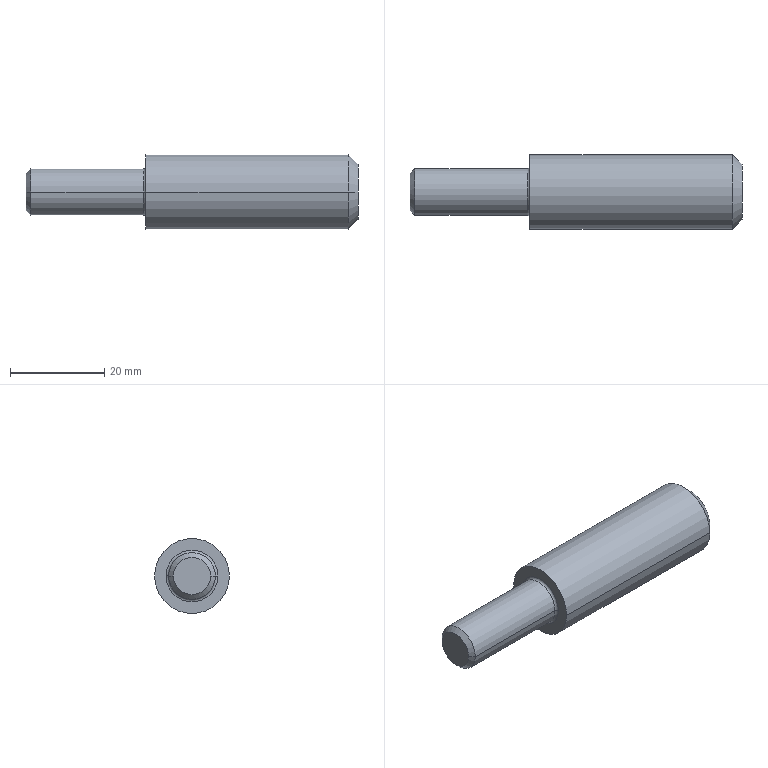Part | NX | features BREP 1 | 1 solid | 13 faces | box 70.358 x 15.875 x 15.875 mm | volume 10759 mm3 | cone 4 | cylinder 4 | plane 3 | torus 2 | commonest cylinder face diameters 9.931 x2 15.875 x2
STEP:
#1=CARTESIAN_POINT('',(0.,-5.905,0.));
#2=VERTEX_POINT('',#1);
#3=CARTESIAN_POINT('',(0.,5.905,0.));
#4=VERTEX_POINT('',#3);
#5=CARTESIAN_POINT('',(0.,0.,0.));
#6=DIRECTION('',(-1.,0.,0.));
#7=DIRECTION('',(0.,-1.,0.));
#8=AXIS2_PLACEMENT_3D('',#5,#6,#7);
#9=CIRCLE('',#8,5.905);
#10=EDGE_CURVE('',#2,#4,#9,.T.);
#11=ORIENTED_EDGE('',*,*,#10,.F.);
#12=CARTESIAN_POINT('',(0.,0.,0.));
#13=DIRECTION('',(-1.,0.,0.));
#14=DIRECTION('',(0.,1.,0.));
#15=AXIS2_PLACEMENT_3D('',#12,#13,#14);
#16=CIRCLE('',#15,5.905);
#17=EDGE_CURVE('',#4,#2,#16,.T.);
#18=ORIENTED_EDGE('',*,*,#17,.F.);
#19=EDGE_LOOP('',(#11,#18));
#20=FACE_BOUND('',#19,.T.);
#21=CARTESIAN_POINT('',(0.,0.,0.));
#22=DIRECTION('',(-1.,0.,0.));
#23=DIRECTION('',(0.,0.,1.));
#24=AXIS2_PLACEMENT_3D('',#21,#22,#23);
#25=PLANE('',#24);
#26=ADVANCED_FACE('',(#20),#25,.F.);
#27=CARTESIAN_POINT('',(-2.032,-7.938,0.));
#28=VERTEX_POINT('',#27);
#29=CARTESIAN_POINT('',(0.,-5.905,0.));
#30=DIRECTION('',(-0.7071,-0.7071,0.));
#31=VECTOR('',#30,1000.);
#32=LINE('',#29,#31);
#33=EDGE_CURVE('',#2,#28,#32,.T.);
#34=ORIENTED_EDGE('',*,*,#33,.T.);
#35=CARTESIAN_POINT('',(-2.032,7.938,0.));
#36=VERTEX_POINT('',#35);
#37=CARTESIAN_POINT('',(-2.032,0.,0.));
#38=DIRECTION('',(-1.,0.,0.));
#39=DIRECTION('',(0.,1.,0.));
#40=AXIS2_PLACEMENT_3D('',#37,#38,#39);
#41=CIRCLE('',#40,7.938);
#42=EDGE_CURVE('',#36,#28,#41,.T.);
#43=ORIENTED_EDGE('',*,*,#42,.F.);
#44=CARTESIAN_POINT('',(0.,5.905,0.));
#45=DIRECTION('',(-0.7071,0.7071,0.));
#46=VECTOR('',#45,1000.);
#47=LINE('',#44,#46);
#48=EDGE_CURVE('',#4,#36,#47,.T.);
#49=ORIENTED_EDGE('',*,*,#48,.F.);
#50=ORIENTED_EDGE('',*,*,#17,.T.);
#51=EDGE_LOOP('',(#34,#43,#49,#50));
#52=FACE_BOUND('',#51,.T.);
#53=CARTESIAN_POINT('',(-1.016,0.,0.));
#54=DIRECTION('',(-1.,0.,0.));
#55=DIRECTION('',(0.,1.,0.));
#56=AXIS2_PLACEMENT_3D('',#53,#54,#55);
#57=CONICAL_SURFACE('',#56,6.921,0.7854);
#58=ADVANCED_FACE('',(#52),#57,.T.);
#59=ORIENTED_EDGE('',*,*,#48,.T.);
#60=CARTESIAN_POINT('',(-2.032,0.,0.));
#61=DIRECTION('',(-1.,0.,0.));
#62=DIRECTION('',(0.,-1.,0.));
#63=AXIS2_PLACEMENT_3D('',#60,#61,#62);
#64=CIRCLE('',#63,7.938);
#65=EDGE_CURVE('',#28,#36,#64,.T.);
#66=ORIENTED_EDGE('',*,*,#65,.F.);
#67=ORIENTED_EDGE('',*,*,#33,.F.);
#68=ORIENTED_EDGE('',*,*,#10,.T.);
#69=EDGE_LOOP('',(#59,#66,#67,#68));
#70=FACE_BOUND('',#69,.T.);
#71=CARTESIAN_POINT('',(-1.016,0.,0.));
#72=DIRECTION('',(-1.,0.,0.));
#73=DIRECTION('',(0.,1.,0.));
#74=AXIS2_PLACEMENT_3D('',#71,#72,#73);
#75=CONICAL_SURFACE('',#74,6.921,0.7854);
#76=ADVANCED_FACE('',(#70),#75,.T.);
#77=CARTESIAN_POINT('',(-44.958,7.938,0.));
#78=VERTEX_POINT('',#77);
#79=CARTESIAN_POINT('',(-2.032,7.938,0.));
#80=DIRECTION('',(-1.,0.,0.));
#81=VECTOR('',#80,1000.);
#82=LINE('',#79,#81);
#83=EDGE_CURVE('',#78,#36,#82,.F.);
#84=ORIENTED_EDGE('',*,*,#83,.F.);
#85=CARTESIAN_POINT('',(-44.958,-7.938,0.));
#86=VERTEX_POINT('',#85);
#87=CARTESIAN_POINT('',(-44.958,0.,0.));
#88=DIRECTION('',(-1.,0.,0.));
#89=DIRECTION('',(0.,-1.,0.));
#90=AXIS2_PLACEMENT_3D('',#87,#88,#89);
#91=CIRCLE('',#90,7.938);
#92=EDGE_CURVE('',#86,#78,#91,.T.);
#93=ORIENTED_EDGE('',*,*,#92,.F.);
#94=CARTESIAN_POINT('',(-2.032,-7.938,0.));
#95=DIRECTION('',(-1.,0.,0.));
#96=VECTOR('',#95,1000.);
#97=LINE('',#94,#96);
#98=EDGE_CURVE('',#86,#28,#97,.F.);
#99=ORIENTED_EDGE('',*,*,#98,.T.);
#100=ORIENTED_EDGE('',*,*,#65,.T.);
#101=EDGE_LOOP('',(#84,#93,#99,#100));
#102=FACE_BOUND('',#101,.T.);
#103=CARTESIAN_POINT('',(0.,0.,0.));
#104=DIRECTION('',(-1.,0.,0.));
#105=DIRECTION('',(0.,1.,0.));
#106=AXIS2_PLACEMENT_3D('',#103,#104,#105);
#107=CYLINDRICAL_SURFACE('',#106,7.938);
#108=ADVANCED_FACE('',(#102),#107,.T.);
#109=ORIENTED_EDGE('',*,*,#98,.F.);
#110=CARTESIAN_POINT('',(-44.958,0.,0.));
#111=DIRECTION('',(-1.,0.,0.));
#112=DIRECTION('',(0.,1.,0.));
#113=AXIS2_PLACEMENT_3D('',#110,#111,#112);
#114=CIRCLE('',#113,7.938);
#115=EDGE_CURVE('',#78,#86,#114,.T.);
#116=ORIENTED_EDGE('',*,*,#115,.F.);
#117=ORIENTED_EDGE('',*,*,#83,.T.);
#118=ORIENTED_EDGE('',*,*,#42,.T.);
#119=EDGE_LOOP('',(#109,#116,#117,#118));
#120=FACE_BOUND('',#119,.T.);
#121=CARTESIAN_POINT('',(0.,0.,0.));
#122=DIRECTION('',(-1.,0.,0.));
#123=DIRECTION('',(0.,1.,0.));
#124=AXIS2_PLACEMENT_3D('',#121,#122,#123);
#125=CYLINDRICAL_SURFACE('',#124,7.938);
#126=ADVANCED_FACE('',(#120),#125,.T.);
#127=ORIENTED_EDGE('',*,*,#92,.T.);
#128=ORIENTED_EDGE('',*,*,#115,.T.);
#129=EDGE_LOOP('',(#127,#128));
#130=FACE_BOUND('',#129,.T.);
#131=CARTESIAN_POINT('',(-44.958,-5.474,0.));
#132=VERTEX_POINT('',#131);
#133=CARTESIAN_POINT('',(-44.958,5.474,0.));
#134=VERTEX_POINT('',#133);
#135=CARTESIAN_POINT('',(-44.958,0.,0.));
#136=DIRECTION('',(-1.,0.,0.));
#137=DIRECTION('',(0.,-1.,0.));
#138=AXIS2_PLACEMENT_3D('',#135,#136,#137);
#139=CIRCLE('',#138,5.474);
#140=EDGE_CURVE('',#132,#134,#139,.T.);
#141=ORIENTED_EDGE('',*,*,#140,.F.);
#142=CARTESIAN_POINT('',(-44.958,0.,0.));
#143=DIRECTION('',(-1.,0.,0.));
#144=DIRECTION('',(0.,1.,0.));
#145=AXIS2_PLACEMENT_3D('',#142,#143,#144);
#146=CIRCLE('',#145,5.474);
#147=EDGE_CURVE('',#134,#132,#146,.T.);
#148=ORIENTED_EDGE('',*,*,#147,.F.);
#149=EDGE_LOOP('',(#141,#148));
#150=FACE_BOUND('',#149,.T.);
#151=CARTESIAN_POINT('',(-44.958,0.,0.));
#152=DIRECTION('',(-1.,0.,0.));
#153=DIRECTION('',(0.,0.,1.));
#154=AXIS2_PLACEMENT_3D('',#151,#152,#153);
#155=PLANE('',#154);
#156=ADVANCED_FACE('',(#130,#150),#155,.T.);
#157=CARTESIAN_POINT('',(-45.466,-4.966,0.));
#158=VERTEX_POINT('',#157);
#159=CARTESIAN_POINT('',(-45.466,-5.474,0.));
#160=DIRECTION('',(0.,0.,1.));
#161=DIRECTION('',(1.,0.,0.));
#162=AXIS2_PLACEMENT_3D('',#159,#160,#161);
#163=CIRCLE('',#162,0.508);
#164=EDGE_CURVE('',#132,#158,#163,.T.);
#165=ORIENTED_EDGE('',*,*,#164,.T.);
#166=CARTESIAN_POINT('',(-45.466,4.966,0.));
#167=VERTEX_POINT('',#166);
#168=CARTESIAN_POINT('',(-45.466,0.,0.));
#169=DIRECTION('',(-1.,0.,0.));
#170=DIRECTION('',(0.,1.,0.));
#171=AXIS2_PLACEMENT_3D('',#168,#169,#170);
#172=CIRCLE('',#171,4.966);
#173=EDGE_CURVE('',#167,#158,#172,.T.);
#174=ORIENTED_EDGE('',*,*,#173,.F.);
#175=CARTESIAN_POINT('',(-45.466,5.474,0.));
#176=DIRECTION('',(0.,0.,-1.));
#177=DIRECTION('',(1.,0.,0.));
#178=AXIS2_PLACEMENT_3D('',#175,#176,#177);
#179=CIRCLE('',#178,0.508);
#180=EDGE_CURVE('',#134,#167,#179,.T.);
#181=ORIENTED_EDGE('',*,*,#180,.F.);
#182=ORIENTED_EDGE('',*,*,#147,.T.);
#183=EDGE_LOOP('',(#165,#174,#181,#182));
#184=FACE_BOUND('',#183,.T.);
#185=CARTESIAN_POINT('',(-45.466,0.,0.));
#186=DIRECTION('',(-1.,0.,0.));
#187=DIRECTION('',(0.,0.9997,0.02287));
#188=AXIS2_PLACEMENT_3D('',#185,#186,#187);
#189=TOROIDAL_SURFACE('',#188,5.474,0.508);
#190=ADVANCED_FACE('',(#184),#189,.F.);
#191=ORIENTED_EDGE('',*,*,#180,.T.);
#192=CARTESIAN_POINT('',(-45.466,0.,0.));
#193=DIRECTION('',(-1.,0.,0.));
#194=DIRECTION('',(0.,-1.,0.));
#195=AXIS2_PLACEMENT_3D('',#192,#193,#194);
#196=CIRCLE('',#195,4.966);
#197=EDGE_CURVE('',#158,#167,#196,.T.);
#198=ORIENTED_EDGE('',*,*,#197,.F.);
#199=ORIENTED_EDGE('',*,*,#164,.F.);
#200=ORIENTED_EDGE('',*,*,#140,.T.);
#201=EDGE_LOOP('',(#191,#198,#199,#200));
#202=FACE_BOUND('',#201,.T.);
#203=CARTESIAN_POINT('',(-45.466,0.,0.));
#204=DIRECTION('',(-1.,0.,0.));
#205=DIRECTION('',(0.,-0.9997,-0.02287));
#206=AXIS2_PLACEMENT_3D('',#203,#204,#205);
#207=TOROIDAL_SURFACE('',#206,5.474,0.508);
#208=ADVANCED_FACE('',(#202),#207,.F.);
#209=CARTESIAN_POINT('',(-69.342,4.966,0.));
#210=VERTEX_POINT('',#209);
#211=CARTESIAN_POINT('',(-45.466,4.966,0.));
#212=DIRECTION('',(-1.,0.,0.));
#213=VECTOR('',#212,1000.);
#214=LINE('',#211,#213);
#215=EDGE_CURVE('',#210,#167,#214,.F.);
#216=ORIENTED_EDGE('',*,*,#215,.F.);
#217=CARTESIAN_POINT('',(-69.342,-4.966,0.));
#218=VERTEX_POINT('',#217);
#219=CARTESIAN_POINT('',(-69.342,0.,0.));
#220=DIRECTION('',(-1.,0.,0.));
#221=DIRECTION('',(0.,-1.,0.));
#222=AXIS2_PLACEMENT_3D('',#219,#220,#221);
#223=CIRCLE('',#222,4.966);
#224=EDGE_CURVE('',#218,#210,#223,.T.);
#225=ORIENTED_EDGE('',*,*,#224,.F.);
#226=CARTESIAN_POINT('',(-45.466,-4.966,0.));
#227=DIRECTION('',(-1.,0.,0.));
#228=VECTOR('',#227,1000.);
#229=LINE('',#226,#228);
#230=EDGE_CURVE('',#218,#158,#229,.F.);
#231=ORIENTED_EDGE('',*,*,#230,.T.);
#232=ORIENTED_EDGE('',*,*,#197,.T.);
#233=EDGE_LOOP('',(#216,#225,#231,#232));
#234=FACE_BOUND('',#233,.T.);
#235=CARTESIAN_POINT('',(-44.958,0.,0.));
#236=DIRECTION('',(-1.,0.,0.));
#237=DIRECTION('',(0.,1.,0.));
#238=AXIS2_PLACEMENT_3D('',#235,#236,#237);
#239=CYLINDRICAL_SURFACE('',#238,4.966);
#240=ADVANCED_FACE('',(#234),#239,.T.);
#241=ORIENTED_EDGE('',*,*,#230,.F.);
#242=CARTESIAN_POINT('',(-69.342,0.,0.));
#243=DIRECTION('',(-1.,0.,0.));
#244=DIRECTION('',(0.,1.,0.));
#245=AXIS2_PLACEMENT_3D('',#242,#243,#244);
#246=CIRCLE('',#245,4.966);
#247=EDGE_CURVE('',#210,#218,#246,.T.);
#248=ORIENTED_EDGE('',*,*,#247,.F.);
#249=ORIENTED_EDGE('',*,*,#215,.T.);
#250=ORIENTED_EDGE('',*,*,#173,.T.);
#251=EDGE_LOOP('',(#241,#248,#249,#250));
#252=FACE_BOUND('',#251,.T.);
#253=CARTESIAN_POINT('',(-44.958,0.,0.));
#254=DIRECTION('',(-1.,0.,0.));
#255=DIRECTION('',(0.,1.,0.));
#256=AXIS2_PLACEMENT_3D('',#253,#254,#255);
#257=CYLINDRICAL_SURFACE('',#256,4.966);
#258=ADVANCED_FACE('',(#252),#257,.T.);
#259=CARTESIAN_POINT('',(-70.358,3.95,0.));
#260=VERTEX_POINT('',#259);
#261=CARTESIAN_POINT('',(-70.358,3.95,0.));
#262=DIRECTION('',(0.7071,0.7071,0.));
#263=VECTOR('',#262,1000.);
#264=LINE('',#261,#263);
#265=EDGE_CURVE('',#210,#260,#264,.F.);
#266=ORIENTED_EDGE('',*,*,#265,.F.);
#267=ORIENTED_EDGE('',*,*,#247,.T.);
#268=CARTESIAN_POINT('',(-70.358,-3.95,0.));
#269=VERTEX_POINT('',#268);
#270=CARTESIAN_POINT('',(-70.358,-3.95,0.));
#271=DIRECTION('',(0.7071,-0.7071,0.));
#272=VECTOR('',#271,1000.);
#273=LINE('',#270,#272);
#274=EDGE_CURVE('',#218,#269,#273,.F.);
#275=ORIENTED_EDGE('',*,*,#274,.T.);
#276=CARTESIAN_POINT('',(-70.358,0.,0.));
#277=DIRECTION('',(-1.,0.,0.));
#278=DIRECTION('',(0.,1.,0.));
#279=AXIS2_PLACEMENT_3D('',#276,#277,#278);
#280=CIRCLE('',#279,3.95);
#281=EDGE_CURVE('',#260,#269,#280,.T.);
#282=ORIENTED_EDGE('',*,*,#281,.F.);
#283=EDGE_LOOP('',(#266,#267,#275,#282));
#284=FACE_BOUND('',#283,.T.);
#285=CARTESIAN_POINT('',(-69.85,0.,0.));
#286=DIRECTION('',(1.,0.,0.));
#287=DIRECTION('',(0.,-1.,0.));
#288=AXIS2_PLACEMENT_3D('',#285,#286,#287);
#289=CONICAL_SURFACE('',#288,4.458,0.7854);
#290=ADVANCED_FACE('',(#284),#289,.T.);
#291=CARTESIAN_POINT('',(-70.358,0.,0.));
#292=DIRECTION('',(-1.,0.,0.));
#293=DIRECTION('',(0.,-1.,0.));
#294=AXIS2_PLACEMENT_3D('',#291,#292,#293);
#295=CIRCLE('',#294,3.95);
#296=EDGE_CURVE('',#269,#260,#295,.T.);
#297=ORIENTED_EDGE('',*,*,#296,.T.);
#298=ORIENTED_EDGE('',*,*,#281,.T.);
#299=EDGE_LOOP('',(#297,#298));
#300=FACE_BOUND('',#299,.T.);
#301=CARTESIAN_POINT('',(-70.358,0.,0.));
#302=DIRECTION('',(-1.,0.,0.));
#303=DIRECTION('',(0.,0.,1.));
#304=AXIS2_PLACEMENT_3D('',#301,#302,#303);
#305=PLANE('',#304);
#306=ADVANCED_FACE('',(#300),#305,.T.);
#307=ORIENTED_EDGE('',*,*,#274,.F.);
#308=ORIENTED_EDGE('',*,*,#224,.T.);
#309=ORIENTED_EDGE('',*,*,#265,.T.);
#310=ORIENTED_EDGE('',*,*,#296,.F.);
#311=EDGE_LOOP('',(#307,#308,#309,#310));
#312=FACE_BOUND('',#311,.T.);
#313=CARTESIAN_POINT('',(-69.85,0.,0.));
#314=DIRECTION('',(1.,0.,0.));
#315=DIRECTION('',(0.,-1.,0.));
#316=AXIS2_PLACEMENT_3D('',#313,#314,#315);
#317=CONICAL_SURFACE('',#316,4.458,0.7854);
#318=ADVANCED_FACE('',(#312),#317,.T.);
#319=CLOSED_SHELL('',(#26,#58,#76,#108,#126,#156,#190,#208,#240,#258,#290,#306,#318));
#320=MANIFOLD_SOLID_BREP('',#319);
#321=(LENGTH_UNIT()NAMED_UNIT(*)SI_UNIT(.MILLI.,.METRE.));
#322=UNCERTAINTY_MEASURE_WITH_UNIT(LENGTH_MEASURE(0.00001),#321,'','');
#323=(NAMED_UNIT(*)PLANE_ANGLE_UNIT()SI_UNIT($,.RADIAN.));
#324=(NAMED_UNIT(*)SI_UNIT($,.STERADIAN.)SOLID_ANGLE_UNIT());
#325=(GEOMETRIC_REPRESENTATION_CONTEXT(3)GLOBAL_UNCERTAINTY_ASSIGNED_CONTEXT((#322))GLOBAL_UNIT_ASSIGNED_CONTEXT((#321,#323,#324))REPRESENTATION_CONTEXT('',''));
#326=ADVANCED_BREP_SHAPE_REPRESENTATION('',(#320),#325);